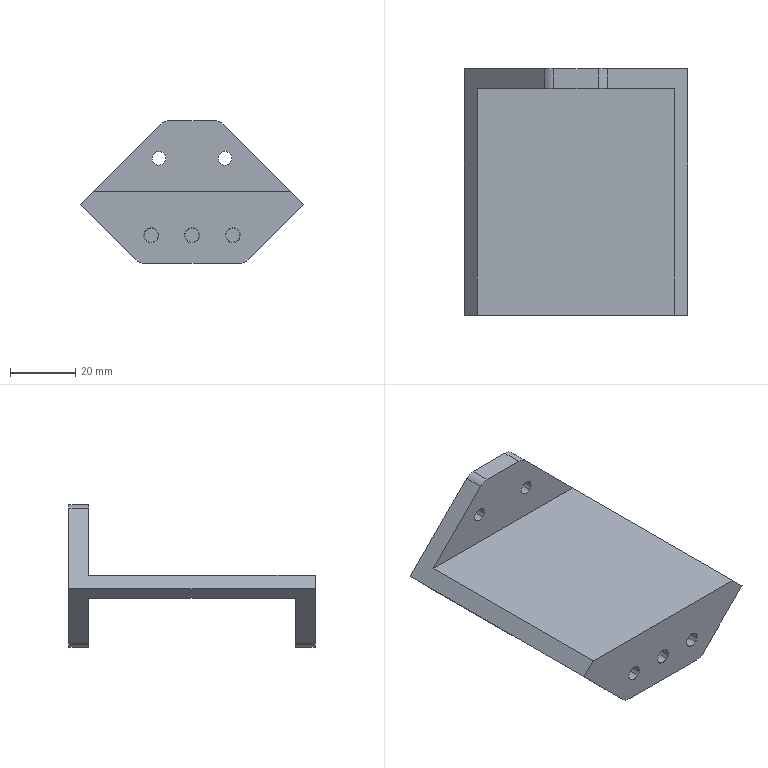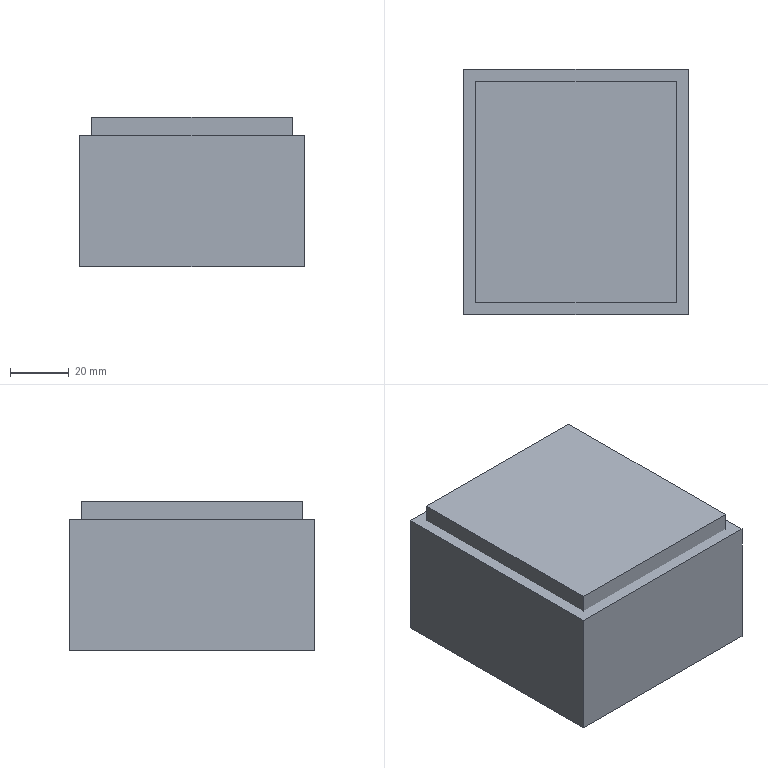CAM job | NX | 3+2 milling, drilling | part box 68.307 x 75.3 x 43.668 mm | stock box 76.307 x 83.3 x 50.668 mm
Tools:
number,name,description,diameter,corner_radius,flute_length,length,flutes
19,D80,Milling Tool-5 Parameters,80.0,0.0,50.0,75.0,2
15,D10,Milling Tool-5 Parameters,10.0,0.0,50.0,75.0,2
14,D10JING,Milling Tool-5 Parameters,10.0,0.0,50.0,75.0,2
16,D6R0.5,Milling Tool-5 Parameters,6.0,0.5,50.0,75.0,2
1,D6A45,Milling Tool-5 Parameters,6.0,0.0,50.0,75.0,2
4,4.2ZT,Drilling Tool,4.2,0.0,35.0,50.0,2
3,D3,Milling Tool-5 Parameters,3.0,0.0,50.0,75.0,2
Operations:
program,operation,operation_type,tool,method,geometry_group,spindle_rpm,surface_speed,feed_per_tooth,feed_cut,feed_plunge,cut_length_mm,path_length_mm,cut_time_min,machine_time_min
1,FLOOR_WALL_COPY,VolumeBased25DMillingOperation,D80,METHOD,A,6500.0,1633.0,0.1154,1500.0,100.0,179.3,233.3,0.1195,0.1249
1,ADAPTIVE_MILLING,CavityMilling,D10,METHOD,A,9500.0,298.0,0.1579,3000.0,1000.0,10497.596,10581.296,3.501,3.51
1,ADAPTIVE_MILLING_COPY,CavityMilling,D10,METHOD,A,9500.0,298.0,0.1579,3000.0,1000.0,2642.051,2907.109,0.8847,0.9112
1,ZLEVEL_PROFILE_1_COPY,ZLevelMilling,D10,METHOD,A,9500.0,119.0,0.1842,3500.0,100.0,4174.074,4820.915,1.193,1.257
1,ZLEVEL_PROFILE_COPY_1_COPY_COPY_1_COPY,ZLevelMilling,D10JING,METHOD,A,9500.0,298.0,0.0632,1200.0,1000.0,977.837,1333.228,0.8166,0.8522
1,FLOOR_WALL_1,VolumeBased25DMillingOperation,D10JING,METHOD,A,9500.0,298.0,0.0658,1250.0,100.0,1100.588,1406.388,0.8805,0.9111
1,ZLEVEL_PROFILE_1,ZLevelMilling,D6R0.5,METHOD,A,9500.0,119.0,0.1842,3500.0,100.0,14516.592,15256.138,4.148,4.222
1,PLANAR_MILL_COPY_COPY_COPY_COPY_COPY_COPY_1_COPY_1,PlanarMilling,D6A45,METHOD,A,9500.0,179.0,0.0658,1250.0,100.0,165.442,480.743,0.1324,0.1639
2,FLOOR_WALL_COPY_COPY,VolumeBased25DMillingOperation,D80,METHOD,B,6500.0,1633.0,0.1154,1500.0,100.0,2491.37,3087.154,1.661,1.72
2,ADAPTIVE_MILLING_COPY_1,CavityMilling,D10,METHOD,B,9500.0,298.0,0.1579,3000.0,1000.0,7418.995,9991.69,2.505,2.762
2,ZLEVEL_PROFILE_1_COPY_COPY,ZLevelMilling,D10,METHOD,B,9500.0,119.0,0.1842,3500.0,100.0,4252.998,4681.294,1.215,1.258
2,FLOOR_WALL_1_COPY,VolumeBased25DMillingOperation,D10JING,METHOD,B,9500.0,298.0,0.0658,1250.0,100.0,1142.395,1337.567,0.9139,0.9334
2,ZLEVEL_PROFILE_1_COPY_1,ZLevelMilling,D6R0.5,METHOD,B,9500.0,119.0,0.1842,3500.0,100.0,14849.724,15226.689,4.243,4.28
2,PLANAR_MILL_COPY_COPY_COPY_COPY_COPY_COPY_1_COPY_1_COPY,PlanarMilling,D6A45,METHOD,B,9500.0,179.0,0.0658,1250.0,100.0,82.721,210.721,0.0662,0.079
2,PLANAR_MILL_COPY_COPY_COPY_COPY_COPY_COPY_1_COPY_1_COPY_COPY,PlanarMilling,D6A45,METHOD,B,9500.0,179.0,0.0658,1250.0,100.0,67.017,169.353,0.0536,0.0638
3,DRILLING_COPY_1_COPY,Operation,D6A45,METHOD,C,5000.0,94.0,0.035,350.0,0.0,16.0,150.987,0.0457,0.0592
3,DRILLING_COPY_1_COPY_1_1_COPY_1,Operation,4.2ZT,METHOD,C,2000.0,34.0,0.05,200.0,0.0,23.524,130.491,0.1176,0.1283
3,HOLE_MILLING,CylinderMilling,D3,METHOD,C,9500.0,89.0,0.0658,1250.0,100.0,120.995,260.995,0.0968,0.1108
3,PLANAR_MILL_COPY_COPY_COPY_COPY_COPY_COPY_1_COPY_1_COPY_1_1,PlanarMilling,D6A45,METHOD,C,9500.0,179.0,0.0658,1250.0,100.0,62.606,325.998,0.0501,0.0764
3,CUTTERCOMP3,CylinderMilling,D3,METHOD,C,9500.0,89.0,0.0526,1000.0,100.0,35.444,175.444,0.0354,0.0494